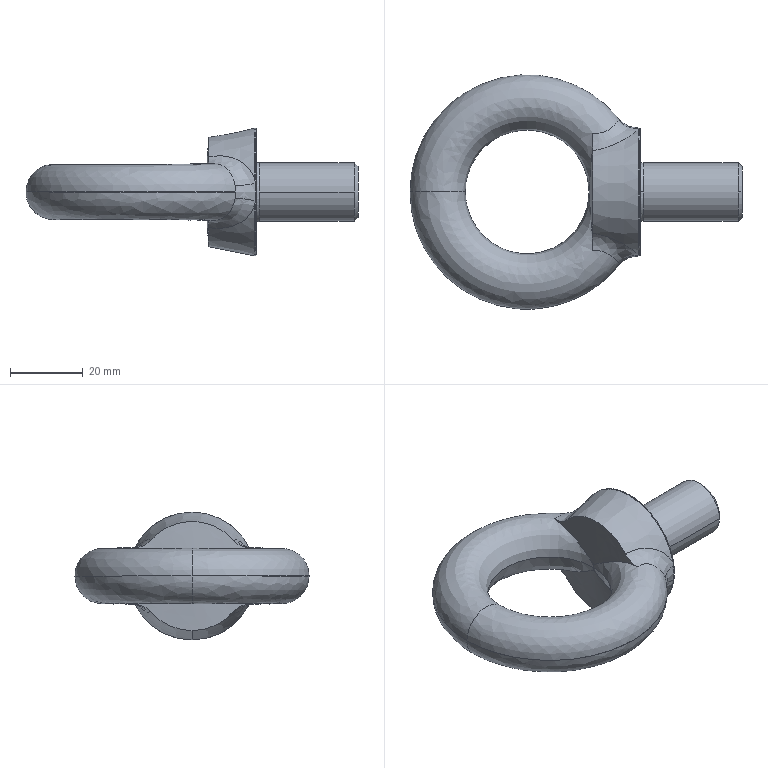Part | SolidWorks | features BaseBody 1 | 1 solid | 37 faces | box 91.2 x 64.4 x 35.09 mm | volume 39752 mm3 | spline 28 | cone 5 | plane 2 | cylinder 2 | commonest cylinder face diameters 16 x2